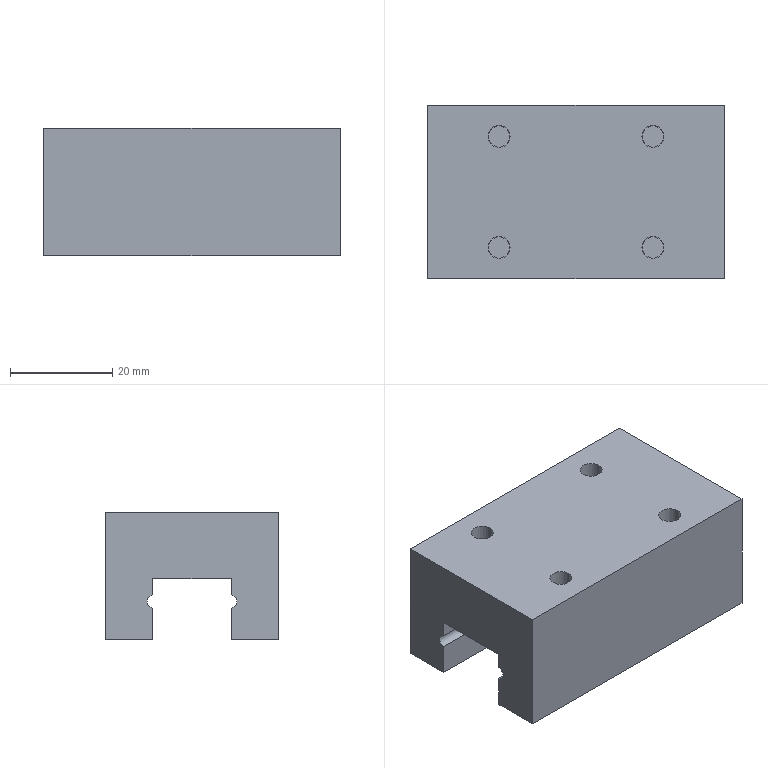Part | SolidWorks | features BaseBody 1 | 1 solid | 38 faces | box 58 x 34 x 25 mm | volume 37485 mm3 | plane 20 | cylinder 18 | commonest cylinder face diameters 4.2 x8 4.3 x8 2.6 x2
STEP:
#1=CARTESIAN_POINT('',(12.93,10.88,21.8));
#2=VERTEX_POINT('',#1);
#3=CARTESIAN_POINT('',(17.23,10.88,21.8));
#4=VERTEX_POINT('',#3);
#5=CARTESIAN_POINT('',(15.08,10.88,21.8));
#6=DIRECTION('',(0.,0.,1.));
#7=DIRECTION('',(1.,0.,0.));
#8=AXIS2_PLACEMENT_3D('',#5,#6,#7);
#9=CIRCLE('',#8,2.15);
#10=EDGE_CURVE('',#2,#4,#9,.T.);
#11=ORIENTED_EDGE('',*,*,#10,.F.);
#12=CARTESIAN_POINT('',(12.93,10.88,28.));
#13=VERTEX_POINT('',#12);
#14=CARTESIAN_POINT('',(12.93,10.88,21.8));
#15=DIRECTION('',(0.,0.,1.));
#16=VECTOR('',#15,1000.);
#17=LINE('',#14,#16);
#18=EDGE_CURVE('',#2,#13,#17,.T.);
#19=ORIENTED_EDGE('',*,*,#18,.T.);
#20=CARTESIAN_POINT('',(17.23,10.88,28.));
#21=VERTEX_POINT('',#20);
#22=CARTESIAN_POINT('',(15.08,10.88,28.));
#23=DIRECTION('',(0.,0.,-1.));
#24=DIRECTION('',(1.,0.,0.));
#25=AXIS2_PLACEMENT_3D('',#22,#23,#24);
#26=CIRCLE('',#25,2.15);
#27=EDGE_CURVE('',#21,#13,#26,.T.);
#28=ORIENTED_EDGE('',*,*,#27,.F.);
#29=CARTESIAN_POINT('',(17.23,10.88,21.8));
#30=DIRECTION('',(0.,0.,1.));
#31=VECTOR('',#30,1000.);
#32=LINE('',#29,#31);
#33=EDGE_CURVE('',#4,#21,#32,.T.);
#34=ORIENTED_EDGE('',*,*,#33,.F.);
#35=EDGE_LOOP('',(#11,#19,#28,#34));
#36=FACE_OUTER_BOUND('',#35,.T.);
#37=CARTESIAN_POINT('',(15.08,10.88,21.8));
#38=DIRECTION('',(0.,0.,1.));
#39=DIRECTION('',(1.,0.,0.));
#40=AXIS2_PLACEMENT_3D('',#37,#38,#39);
#41=CYLINDRICAL_SURFACE('',#40,2.15);
#42=ADVANCED_FACE('',(#36),#41,.F.);
#43=CARTESIAN_POINT('',(-17.23,10.88,21.8));
#44=VERTEX_POINT('',#43);
#45=CARTESIAN_POINT('',(-12.93,10.88,21.8));
#46=VERTEX_POINT('',#45);
#47=CARTESIAN_POINT('',(-15.08,10.88,21.8));
#48=DIRECTION('',(0.,0.,1.));
#49=DIRECTION('',(1.,0.,0.));
#50=AXIS2_PLACEMENT_3D('',#47,#48,#49);
#51=CIRCLE('',#50,2.15);
#52=EDGE_CURVE('',#44,#46,#51,.T.);
#53=ORIENTED_EDGE('',*,*,#52,.F.);
#54=CARTESIAN_POINT('',(-17.23,10.88,28.));
#55=VERTEX_POINT('',#54);
#56=CARTESIAN_POINT('',(-17.23,10.88,21.8));
#57=DIRECTION('',(0.,0.,1.));
#58=VECTOR('',#57,1000.);
#59=LINE('',#56,#58);
#60=EDGE_CURVE('',#44,#55,#59,.T.);
#61=ORIENTED_EDGE('',*,*,#60,.T.);
#62=CARTESIAN_POINT('',(-12.93,10.88,28.));
#63=VERTEX_POINT('',#62);
#64=CARTESIAN_POINT('',(-15.08,10.88,28.));
#65=DIRECTION('',(0.,0.,-1.));
#66=DIRECTION('',(1.,0.,0.));
#67=AXIS2_PLACEMENT_3D('',#64,#65,#66);
#68=CIRCLE('',#67,2.15);
#69=EDGE_CURVE('',#63,#55,#68,.T.);
#70=ORIENTED_EDGE('',*,*,#69,.F.);
#71=CARTESIAN_POINT('',(-12.93,10.88,21.8));
#72=DIRECTION('',(0.,0.,1.));
#73=VECTOR('',#72,1000.);
#74=LINE('',#71,#73);
#75=EDGE_CURVE('',#46,#63,#74,.T.);
#76=ORIENTED_EDGE('',*,*,#75,.F.);
#77=EDGE_LOOP('',(#53,#61,#70,#76));
#78=FACE_OUTER_BOUND('',#77,.T.);
#79=CARTESIAN_POINT('',(-15.08,10.88,21.8));
#80=DIRECTION('',(0.,0.,1.));
#81=DIRECTION('',(1.,0.,0.));
#82=AXIS2_PLACEMENT_3D('',#79,#80,#81);
#83=CYLINDRICAL_SURFACE('',#82,2.15);
#84=ADVANCED_FACE('',(#78),#83,.F.);
#85=CARTESIAN_POINT('',(12.93,-10.88,21.8));
#86=VERTEX_POINT('',#85);
#87=CARTESIAN_POINT('',(17.23,-10.88,21.8));
#88=VERTEX_POINT('',#87);
#89=CARTESIAN_POINT('',(15.08,-10.88,21.8));
#90=DIRECTION('',(0.,0.,1.));
#91=DIRECTION('',(1.,0.,0.));
#92=AXIS2_PLACEMENT_3D('',#89,#90,#91);
#93=CIRCLE('',#92,2.15);
#94=EDGE_CURVE('',#86,#88,#93,.T.);
#95=ORIENTED_EDGE('',*,*,#94,.F.);
#96=CARTESIAN_POINT('',(12.93,-10.88,28.));
#97=VERTEX_POINT('',#96);
#98=CARTESIAN_POINT('',(12.93,-10.88,21.8));
#99=DIRECTION('',(0.,0.,1.));
#100=VECTOR('',#99,1000.);
#101=LINE('',#98,#100);
#102=EDGE_CURVE('',#86,#97,#101,.T.);
#103=ORIENTED_EDGE('',*,*,#102,.T.);
#104=CARTESIAN_POINT('',(17.23,-10.88,28.));
#105=VERTEX_POINT('',#104);
#106=CARTESIAN_POINT('',(15.08,-10.88,28.));
#107=DIRECTION('',(0.,0.,-1.));
#108=DIRECTION('',(1.,0.,0.));
#109=AXIS2_PLACEMENT_3D('',#106,#107,#108);
#110=CIRCLE('',#109,2.15);
#111=EDGE_CURVE('',#105,#97,#110,.T.);
#112=ORIENTED_EDGE('',*,*,#111,.F.);
#113=CARTESIAN_POINT('',(17.23,-10.88,21.8));
#114=DIRECTION('',(0.,0.,1.));
#115=VECTOR('',#114,1000.);
#116=LINE('',#113,#115);
#117=EDGE_CURVE('',#88,#105,#116,.T.);
#118=ORIENTED_EDGE('',*,*,#117,.F.);
#119=EDGE_LOOP('',(#95,#103,#112,#118));
#120=FACE_OUTER_BOUND('',#119,.T.);
#121=CARTESIAN_POINT('',(15.08,-10.88,21.8));
#122=DIRECTION('',(0.,0.,1.));
#123=DIRECTION('',(1.,0.,0.));
#124=AXIS2_PLACEMENT_3D('',#121,#122,#123);
#125=CYLINDRICAL_SURFACE('',#124,2.15);
#126=ADVANCED_FACE('',(#120),#125,.F.);
#127=CARTESIAN_POINT('',(-17.23,-10.88,21.8));
#128=VERTEX_POINT('',#127);
#129=CARTESIAN_POINT('',(-12.93,-10.88,21.8));
#130=VERTEX_POINT('',#129);
#131=CARTESIAN_POINT('',(-15.08,-10.88,21.8));
#132=DIRECTION('',(0.,0.,1.));
#133=DIRECTION('',(1.,0.,0.));
#134=AXIS2_PLACEMENT_3D('',#131,#132,#133);
#135=CIRCLE('',#134,2.15);
#136=EDGE_CURVE('',#128,#130,#135,.T.);
#137=ORIENTED_EDGE('',*,*,#136,.F.);
#138=CARTESIAN_POINT('',(-17.23,-10.88,28.));
#139=VERTEX_POINT('',#138);
#140=CARTESIAN_POINT('',(-17.23,-10.88,21.8));
#141=DIRECTION('',(0.,0.,1.));
#142=VECTOR('',#141,1000.);
#143=LINE('',#140,#142);
#144=EDGE_CURVE('',#128,#139,#143,.T.);
#145=ORIENTED_EDGE('',*,*,#144,.T.);
#146=CARTESIAN_POINT('',(-12.93,-10.88,28.));
#147=VERTEX_POINT('',#146);
#148=CARTESIAN_POINT('',(-15.08,-10.88,28.));
#149=DIRECTION('',(0.,0.,-1.));
#150=DIRECTION('',(1.,0.,0.));
#151=AXIS2_PLACEMENT_3D('',#148,#149,#150);
#152=CIRCLE('',#151,2.15);
#153=EDGE_CURVE('',#147,#139,#152,.T.);
#154=ORIENTED_EDGE('',*,*,#153,.F.);
#155=CARTESIAN_POINT('',(-12.93,-10.88,21.8));
#156=DIRECTION('',(0.,0.,1.));
#157=VECTOR('',#156,1000.);
#158=LINE('',#155,#157);
#159=EDGE_CURVE('',#130,#147,#158,.T.);
#160=ORIENTED_EDGE('',*,*,#159,.F.);
#161=EDGE_LOOP('',(#137,#145,#154,#160));
#162=FACE_OUTER_BOUND('',#161,.T.);
#163=CARTESIAN_POINT('',(-15.08,-10.88,21.8));
#164=DIRECTION('',(0.,0.,1.));
#165=DIRECTION('',(1.,0.,0.));
#166=AXIS2_PLACEMENT_3D('',#163,#164,#165);
#167=CYLINDRICAL_SURFACE('',#166,2.15);
#168=ADVANCED_FACE('',(#162),#167,.F.);
#169=CARTESIAN_POINT('',(12.98,10.88,12.));
#170=VERTEX_POINT('',#169);
#171=CARTESIAN_POINT('',(17.18,10.88,12.));
#172=VERTEX_POINT('',#171);
#173=CARTESIAN_POINT('',(15.08,10.88,12.));
#174=DIRECTION('',(0.,0.,1.));
#175=DIRECTION('',(1.,0.,0.));
#176=AXIS2_PLACEMENT_3D('',#173,#174,#175);
#177=CIRCLE('',#176,2.1);
#178=EDGE_CURVE('',#170,#172,#177,.T.);
#179=ORIENTED_EDGE('',*,*,#178,.F.);
#180=CARTESIAN_POINT('',(12.98,10.88,21.8));
#181=VERTEX_POINT('',#180);
#182=CARTESIAN_POINT('',(12.98,10.88,12.));
#183=DIRECTION('',(0.,0.,1.));
#184=VECTOR('',#183,1000.);
#185=LINE('',#182,#184);
#186=EDGE_CURVE('',#170,#181,#185,.T.);
#187=ORIENTED_EDGE('',*,*,#186,.T.);
#188=CARTESIAN_POINT('',(17.18,10.88,21.8));
#189=VERTEX_POINT('',#188);
#190=CARTESIAN_POINT('',(15.08,10.88,21.8));
#191=DIRECTION('',(0.,0.,-1.));
#192=DIRECTION('',(1.,0.,0.));
#193=AXIS2_PLACEMENT_3D('',#190,#191,#192);
#194=CIRCLE('',#193,2.1);
#195=EDGE_CURVE('',#189,#181,#194,.T.);
#196=ORIENTED_EDGE('',*,*,#195,.F.);
#197=CARTESIAN_POINT('',(17.18,10.88,12.));
#198=DIRECTION('',(0.,0.,1.));
#199=VECTOR('',#198,1000.);
#200=LINE('',#197,#199);
#201=EDGE_CURVE('',#172,#189,#200,.T.);
#202=ORIENTED_EDGE('',*,*,#201,.F.);
#203=EDGE_LOOP('',(#179,#187,#196,#202));
#204=FACE_OUTER_BOUND('',#203,.T.);
#205=CARTESIAN_POINT('',(15.08,10.88,12.));
#206=DIRECTION('',(0.,0.,1.));
#207=DIRECTION('',(1.,0.,0.));
#208=AXIS2_PLACEMENT_3D('',#205,#206,#207);
#209=CYLINDRICAL_SURFACE('',#208,2.1);
#210=ADVANCED_FACE('',(#204),#209,.F.);
#211=CARTESIAN_POINT('',(-17.18,10.88,12.));
#212=VERTEX_POINT('',#211);
#213=CARTESIAN_POINT('',(-12.98,10.88,12.));
#214=VERTEX_POINT('',#213);
#215=CARTESIAN_POINT('',(-15.08,10.88,12.));
#216=DIRECTION('',(0.,0.,1.));
#217=DIRECTION('',(1.,0.,0.));
#218=AXIS2_PLACEMENT_3D('',#215,#216,#217);
#219=CIRCLE('',#218,2.1);
#220=EDGE_CURVE('',#212,#214,#219,.T.);
#221=ORIENTED_EDGE('',*,*,#220,.F.);
#222=CARTESIAN_POINT('',(-17.18,10.88,21.8));
#223=VERTEX_POINT('',#222);
#224=CARTESIAN_POINT('',(-17.18,10.88,12.));
#225=DIRECTION('',(0.,0.,1.));
#226=VECTOR('',#225,1000.);
#227=LINE('',#224,#226);
#228=EDGE_CURVE('',#212,#223,#227,.T.);
#229=ORIENTED_EDGE('',*,*,#228,.T.);
#230=CARTESIAN_POINT('',(-12.98,10.88,21.8));
#231=VERTEX_POINT('',#230);
#232=CARTESIAN_POINT('',(-15.08,10.88,21.8));
#233=DIRECTION('',(0.,0.,-1.));
#234=DIRECTION('',(1.,0.,0.));
#235=AXIS2_PLACEMENT_3D('',#232,#233,#234);
#236=CIRCLE('',#235,2.1);
#237=EDGE_CURVE('',#231,#223,#236,.T.);
#238=ORIENTED_EDGE('',*,*,#237,.F.);
#239=CARTESIAN_POINT('',(-12.98,10.88,12.));
#240=DIRECTION('',(0.,0.,1.));
#241=VECTOR('',#240,1000.);
#242=LINE('',#239,#241);
#243=EDGE_CURVE('',#214,#231,#242,.T.);
#244=ORIENTED_EDGE('',*,*,#243,.F.);
#245=EDGE_LOOP('',(#221,#229,#238,#244));
#246=FACE_OUTER_BOUND('',#245,.T.);
#247=CARTESIAN_POINT('',(-15.08,10.88,12.));
#248=DIRECTION('',(0.,0.,1.));
#249=DIRECTION('',(1.,0.,0.));
#250=AXIS2_PLACEMENT_3D('',#247,#248,#249);
#251=CYLINDRICAL_SURFACE('',#250,2.1);
#252=ADVANCED_FACE('',(#246),#251,.F.);
#253=CARTESIAN_POINT('',(12.98,-10.88,12.));
#254=VERTEX_POINT('',#253);
#255=CARTESIAN_POINT('',(17.18,-10.88,12.));
#256=VERTEX_POINT('',#255);
#257=CARTESIAN_POINT('',(15.08,-10.88,12.));
#258=DIRECTION('',(0.,0.,1.));
#259=DIRECTION('',(1.,0.,0.));
#260=AXIS2_PLACEMENT_3D('',#257,#258,#259);
#261=CIRCLE('',#260,2.1);
#262=EDGE_CURVE('',#254,#256,#261,.T.);
#263=ORIENTED_EDGE('',*,*,#262,.F.);
#264=CARTESIAN_POINT('',(12.98,-10.88,21.8));
#265=VERTEX_POINT('',#264);
#266=CARTESIAN_POINT('',(12.98,-10.88,12.));
#267=DIRECTION('',(0.,0.,1.));
#268=VECTOR('',#267,1000.);
#269=LINE('',#266,#268);
#270=EDGE_CURVE('',#254,#265,#269,.T.);
#271=ORIENTED_EDGE('',*,*,#270,.T.);
#272=CARTESIAN_POINT('',(17.18,-10.88,21.8));
#273=VERTEX_POINT('',#272);
#274=CARTESIAN_POINT('',(15.08,-10.88,21.8));
#275=DIRECTION('',(0.,0.,-1.));
#276=DIRECTION('',(1.,0.,0.));
#277=AXIS2_PLACEMENT_3D('',#274,#275,#276);
#278=CIRCLE('',#277,2.1);
#279=EDGE_CURVE('',#273,#265,#278,.T.);
#280=ORIENTED_EDGE('',*,*,#279,.F.);
#281=CARTESIAN_POINT('',(17.18,-10.88,12.));
#282=DIRECTION('',(0.,0.,1.));
#283=VECTOR('',#282,1000.);
#284=LINE('',#281,#283);
#285=EDGE_CURVE('',#256,#273,#284,.T.);
#286=ORIENTED_EDGE('',*,*,#285,.F.);
#287=EDGE_LOOP('',(#263,#271,#280,#286));
#288=FACE_OUTER_BOUND('',#287,.T.);
#289=CARTESIAN_POINT('',(15.08,-10.88,12.));
#290=DIRECTION('',(0.,0.,1.));
#291=DIRECTION('',(1.,0.,0.));
#292=AXIS2_PLACEMENT_3D('',#289,#290,#291);
#293=CYLINDRICAL_SURFACE('',#292,2.1);
#294=ADVANCED_FACE('',(#288),#293,.F.);
#295=CARTESIAN_POINT('',(-17.18,-10.88,12.));
#296=VERTEX_POINT('',#295);
#297=CARTESIAN_POINT('',(-12.98,-10.88,12.));
#298=VERTEX_POINT('',#297);
#299=CARTESIAN_POINT('',(-15.08,-10.88,12.));
#300=DIRECTION('',(0.,0.,1.));
#301=DIRECTION('',(1.,0.,0.));
#302=AXIS2_PLACEMENT_3D('',#299,#300,#301);
#303=CIRCLE('',#302,2.1);
#304=EDGE_CURVE('',#296,#298,#303,.T.);
#305=ORIENTED_EDGE('',*,*,#304,.F.);
#306=CARTESIAN_POINT('',(-17.18,-10.88,21.8));
#307=VERTEX_POINT('',#306);
#308=CARTESIAN_POINT('',(-17.18,-10.88,12.));
#309=DIRECTION('',(0.,0.,1.));
#310=VECTOR('',#309,1000.);
#311=LINE('',#308,#310);
#312=EDGE_CURVE('',#296,#307,#311,.T.);
#313=ORIENTED_EDGE('',*,*,#312,.T.);
#314=CARTESIAN_POINT('',(-12.98,-10.88,21.8));
#315=VERTEX_POINT('',#314);
#316=CARTESIAN_POINT('',(-15.08,-10.88,21.8));
#317=DIRECTION('',(0.,0.,-1.));
#318=DIRECTION('',(1.,0.,0.));
#319=AXIS2_PLACEMENT_3D('',#316,#317,#318);
#320=CIRCLE('',#319,2.1);
#321=EDGE_CURVE('',#315,#307,#320,.T.);
#322=ORIENTED_EDGE('',*,*,#321,.F.);
#323=CARTESIAN_POINT('',(-12.98,-10.88,12.));
#324=DIRECTION('',(0.,0.,1.));
#325=VECTOR('',#324,1000.);
#326=LINE('',#323,#325);
#327=EDGE_CURVE('',#298,#315,#326,.T.);
#328=ORIENTED_EDGE('',*,*,#327,.F.);
#329=EDGE_LOOP('',(#305,#313,#322,#328));
#330=FACE_OUTER_BOUND('',#329,.T.);
#331=CARTESIAN_POINT('',(-15.08,-10.88,12.));
#332=DIRECTION('',(0.,0.,1.));
#333=DIRECTION('',(1.,0.,0.));
#334=AXIS2_PLACEMENT_3D('',#331,#332,#333);
#335=CYLINDRICAL_SURFACE('',#334,2.1);
#336=ADVANCED_FACE('',(#330),#335,.F.);
#337=ORIENTED_EDGE('',*,*,#27,.T.);
#338=CARTESIAN_POINT('',(15.08,10.88,28.));
#339=DIRECTION('',(0.,0.,-1.));
#340=DIRECTION('',(1.,0.,0.));
#341=AXIS2_PLACEMENT_3D('',#338,#339,#340);
#342=CIRCLE('',#341,2.15);
#343=EDGE_CURVE('',#13,#21,#342,.T.);
#344=ORIENTED_EDGE('',*,*,#343,.T.);
#345=EDGE_LOOP('',(#337,#344));
#346=FACE_BOUND('',#345,.T.);
#347=ORIENTED_EDGE('',*,*,#69,.T.);
#348=CARTESIAN_POINT('',(-15.08,10.88,28.));
#349=DIRECTION('',(0.,0.,-1.));
#350=DIRECTION('',(1.,0.,0.));
#351=AXIS2_PLACEMENT_3D('',#348,#349,#350);
#352=CIRCLE('',#351,2.15);
#353=EDGE_CURVE('',#55,#63,#352,.T.);
#354=ORIENTED_EDGE('',*,*,#353,.T.);
#355=EDGE_LOOP('',(#347,#354));
#356=FACE_BOUND('',#355,.T.);
#357=ORIENTED_EDGE('',*,*,#111,.T.);
#358=CARTESIAN_POINT('',(15.08,-10.88,28.));
#359=DIRECTION('',(0.,0.,-1.));
#360=DIRECTION('',(1.,0.,0.));
#361=AXIS2_PLACEMENT_3D('',#358,#359,#360);
#362=CIRCLE('',#361,2.15);
#363=EDGE_CURVE('',#97,#105,#362,.T.);
#364=ORIENTED_EDGE('',*,*,#363,.T.);
#365=EDGE_LOOP('',(#357,#364));
#366=FACE_BOUND('',#365,.T.);
#367=ORIENTED_EDGE('',*,*,#153,.T.);
#368=CARTESIAN_POINT('',(-15.08,-10.88,28.));
#369=DIRECTION('',(0.,0.,-1.));
#370=DIRECTION('',(1.,0.,0.));
#371=AXIS2_PLACEMENT_3D('',#368,#369,#370);
#372=CIRCLE('',#371,2.15);
#373=EDGE_CURVE('',#139,#147,#372,.T.);
#374=ORIENTED_EDGE('',*,*,#373,.T.);
#375=EDGE_LOOP('',(#367,#374));
#376=FACE_BOUND('',#375,.T.);
#377=CARTESIAN_POINT('',(29.,-17.,28.));
#378=VERTEX_POINT('',#377);
#379=CARTESIAN_POINT('',(29.,17.,28.));
#380=VERTEX_POINT('',#379);
#381=CARTESIAN_POINT('',(29.,-17.,28.));
#382=DIRECTION('',(0.,1.,0.));
#383=VECTOR('',#382,1000.);
#384=LINE('',#381,#383);
#385=EDGE_CURVE('',#378,#380,#384,.T.);
#386=ORIENTED_EDGE('',*,*,#385,.T.);
#387=CARTESIAN_POINT('',(-29.,17.,28.));
#388=VERTEX_POINT('',#387);
#389=CARTESIAN_POINT('',(-29.,17.,28.));
#390=DIRECTION('',(-1.,0.,0.));
#391=VECTOR('',#390,1000.);
#392=LINE('',#389,#391);
#393=EDGE_CURVE('',#380,#388,#392,.T.);
#394=ORIENTED_EDGE('',*,*,#393,.T.);
#395=CARTESIAN_POINT('',(-29.,-17.,28.));
#396=VERTEX_POINT('',#395);
#397=CARTESIAN_POINT('',(-29.,-17.,28.));
#398=DIRECTION('',(0.,-1.,0.));
#399=VECTOR('',#398,1000.);
#400=LINE('',#397,#399);
#401=EDGE_CURVE('',#388,#396,#400,.T.);
#402=ORIENTED_EDGE('',*,*,#401,.T.);
#403=CARTESIAN_POINT('',(-29.,-17.,28.));
#404=DIRECTION('',(1.,0.,0.));
#405=VECTOR('',#404,1000.);
#406=LINE('',#403,#405);
#407=EDGE_CURVE('',#396,#378,#406,.T.);
#408=ORIENTED_EDGE('',*,*,#407,.T.);
#409=EDGE_LOOP('',(#386,#394,#402,#408));
#410=FACE_OUTER_BOUND('',#409,.T.);
#411=CARTESIAN_POINT('',(-29.,-17.,28.));
#412=DIRECTION('',(0.,0.,1.));
#413=DIRECTION('',(1.,0.,0.));
#414=AXIS2_PLACEMENT_3D('',#411,#412,#413);
#415=PLANE('',#414);
#416=ADVANCED_FACE('',(#346,#356,#366,#376,#410),#415,.T.);
#417=ORIENTED_EDGE('',*,*,#18,.F.);
#418=CARTESIAN_POINT('',(15.08,10.88,21.8));
#419=DIRECTION('',(0.,0.,1.));
#420=DIRECTION('',(1.,0.,0.));
#421=AXIS2_PLACEMENT_3D('',#418,#419,#420);
#422=CIRCLE('',#421,2.15);
#423=EDGE_CURVE('',#4,#2,#422,.T.);
#424=ORIENTED_EDGE('',*,*,#423,.F.);
#425=ORIENTED_EDGE('',*,*,#33,.T.);
#426=ORIENTED_EDGE('',*,*,#343,.F.);
#427=EDGE_LOOP('',(#417,#424,#425,#426));
#428=FACE_OUTER_BOUND('',#427,.T.);
#429=CARTESIAN_POINT('',(15.08,10.88,21.8));
#430=DIRECTION('',(0.,0.,1.));
#431=DIRECTION('',(1.,0.,0.));
#432=AXIS2_PLACEMENT_3D('',#429,#430,#431);
#433=CYLINDRICAL_SURFACE('',#432,2.15);
#434=ADVANCED_FACE('',(#428),#433,.F.);
#435=ORIENTED_EDGE('',*,*,#60,.F.);
#436=CARTESIAN_POINT('',(-15.08,10.88,21.8));
#437=DIRECTION('',(0.,0.,1.));
#438=DIRECTION('',(1.,0.,0.));
#439=AXIS2_PLACEMENT_3D('',#436,#437,#438);
#440=CIRCLE('',#439,2.15);
#441=EDGE_CURVE('',#46,#44,#440,.T.);
#442=ORIENTED_EDGE('',*,*,#441,.F.);
#443=ORIENTED_EDGE('',*,*,#75,.T.);
#444=ORIENTED_EDGE('',*,*,#353,.F.);
#445=EDGE_LOOP('',(#435,#442,#443,#444));
#446=FACE_OUTER_BOUND('',#445,.T.);
#447=CARTESIAN_POINT('',(-15.08,10.88,21.8));
#448=DIRECTION('',(0.,0.,1.));
#449=DIRECTION('',(1.,0.,0.));
#450=AXIS2_PLACEMENT_3D('',#447,#448,#449);
#451=CYLINDRICAL_SURFACE('',#450,2.15);
#452=ADVANCED_FACE('',(#446),#451,.F.);
#453=ORIENTED_EDGE('',*,*,#102,.F.);
#454=CARTESIAN_POINT('',(15.08,-10.88,21.8));
#455=DIRECTION('',(0.,0.,1.));
#456=DIRECTION('',(1.,0.,0.));
#457=AXIS2_PLACEMENT_3D('',#454,#455,#456);
#458=CIRCLE('',#457,2.15);
#459=EDGE_CURVE('',#88,#86,#458,.T.);
#460=ORIENTED_EDGE('',*,*,#459,.F.);
#461=ORIENTED_EDGE('',*,*,#117,.T.);
#462=ORIENTED_EDGE('',*,*,#363,.F.);
#463=EDGE_LOOP('',(#453,#460,#461,#462));
#464=FACE_OUTER_BOUND('',#463,.T.);
#465=CARTESIAN_POINT('',(15.08,-10.88,21.8));
#466=DIRECTION('',(0.,0.,1.));
#467=DIRECTION('',(1.,0.,0.));
#468=AXIS2_PLACEMENT_3D('',#465,#466,#467);
#469=CYLINDRICAL_SURFACE('',#468,2.15);
#470=ADVANCED_FACE('',(#464),#469,.F.);
#471=ORIENTED_EDGE('',*,*,#144,.F.);
#472=CARTESIAN_POINT('',(-15.08,-10.88,21.8));
#473=DIRECTION('',(0.,0.,1.));
#474=DIRECTION('',(1.,0.,0.));
#475=AXIS2_PLACEMENT_3D('',#472,#473,#474);
#476=CIRCLE('',#475,2.15);
#477=EDGE_CURVE('',#130,#128,#476,.T.);
#478=ORIENTED_EDGE('',*,*,#477,.F.);
#479=ORIENTED_EDGE('',*,*,#159,.T.);
#480=ORIENTED_EDGE('',*,*,#373,.F.);
#481=EDGE_LOOP('',(#471,#478,#479,#480));
#482=FACE_OUTER_BOUND('',#481,.T.);
#483=CARTESIAN_POINT('',(-15.08,-10.88,21.8));
#484=DIRECTION('',(0.,0.,1.));
#485=DIRECTION('',(1.,0.,0.));
#486=AXIS2_PLACEMENT_3D('',#483,#484,#485);
#487=CYLINDRICAL_SURFACE('',#486,2.15);
#488=ADVANCED_FACE('',(#482),#487,.F.);
#489=ORIENTED_EDGE('',*,*,#393,.F.);
#490=CARTESIAN_POINT('',(29.,17.,3.));
#491=VERTEX_POINT('',#490);
#492=CARTESIAN_POINT('',(29.,17.,3.));
#493=DIRECTION('',(0.,0.,-1.));
#494=VECTOR('',#493,1000.);
#495=LINE('',#492,#494);
#496=EDGE_CURVE('',#380,#491,#495,.T.);
#497=ORIENTED_EDGE('',*,*,#496,.T.);
#498=CARTESIAN_POINT('',(-29.,17.,3.));
#499=VERTEX_POINT('',#498);
#500=CARTESIAN_POINT('',(-29.,17.,3.));
#501=DIRECTION('',(-1.,0.,0.));
#502=VECTOR('',#501,1000.);
#503=LINE('',#500,#502);
#504=EDGE_CURVE('',#491,#499,#503,.T.);
#505=ORIENTED_EDGE('',*,*,#504,.T.);
#506=CARTESIAN_POINT('',(-29.,17.,3.));
#507=DIRECTION('',(0.,0.,1.));
#508=VECTOR('',#507,1000.);
#509=LINE('',#506,#508);
#510=EDGE_CURVE('',#499,#388,#509,.T.);
#511=ORIENTED_EDGE('',*,*,#510,.T.);
#512=EDGE_LOOP('',(#489,#497,#505,#511));
#513=FACE_OUTER_BOUND('',#512,.T.);
#514=CARTESIAN_POINT('',(-29.,17.,3.));
#515=DIRECTION('',(0.,1.,0.));
#516=DIRECTION('',(0.,0.,1.));
#517=AXIS2_PLACEMENT_3D('',#514,#515,#516);
#518=PLANE('',#517);
#519=ADVANCED_FACE('',(#513),#518,.T.);
#520=CARTESIAN_POINT('',(29.,7.65,9.209));
#521=VERTEX_POINT('',#520);
#522=CARTESIAN_POINT('',(29.,7.65,3.));
#523=VERTEX_POINT('',#522);
#524=CARTESIAN_POINT('',(29.,7.65,3.));
#525=DIRECTION('',(0.,0.,-1.));
#526=VECTOR('',#525,1000.);
#527=LINE('',#524,#526);
#528=EDGE_CURVE('',#521,#523,#527,.T.);
#529=ORIENTED_EDGE('',*,*,#528,.T.);
#530=CARTESIAN_POINT('',(29.,-17.,3.));
#531=DIRECTION('',(0.,1.,0.));
#532=VECTOR('',#531,1000.);
#533=LINE('',#530,#532);
#534=EDGE_CURVE('',#523,#491,#533,.T.);
#535=ORIENTED_EDGE('',*,*,#534,.T.);
#536=ORIENTED_EDGE('',*,*,#496,.F.);
#537=ORIENTED_EDGE('',*,*,#385,.F.);
#538=CARTESIAN_POINT('',(29.,-17.,3.));
#539=VERTEX_POINT('',#538);
#540=CARTESIAN_POINT('',(29.,-17.,3.));
#541=DIRECTION('',(0.,0.,-1.));
#542=VECTOR('',#541,1000.);
#543=LINE('',#540,#542);
#544=EDGE_CURVE('',#378,#539,#543,.T.);
#545=ORIENTED_EDGE('',*,*,#544,.T.);
#546=CARTESIAN_POINT('',(29.,-7.65,3.));
#547=VERTEX_POINT('',#546);
#548=CARTESIAN_POINT('',(29.,-17.,3.));
#549=DIRECTION('',(0.,1.,0.));
#550=VECTOR('',#549,1000.);
#551=LINE('',#548,#550);
#552=EDGE_CURVE('',#539,#547,#551,.T.);
#553=ORIENTED_EDGE('',*,*,#552,.T.);
#554=CARTESIAN_POINT('',(29.,-7.65,9.209));
#555=VERTEX_POINT('',#554);
#556=CARTESIAN_POINT('',(29.,-7.65,3.));
#557=DIRECTION('',(0.,0.,1.));
#558=VECTOR('',#557,1000.);
#559=LINE('',#556,#558);
#560=EDGE_CURVE('',#547,#555,#559,.T.);
#561=ORIENTED_EDGE('',*,*,#560,.T.);
#562=CARTESIAN_POINT('',(29.,-7.65,11.791));
#563=VERTEX_POINT('',#562);
#564=CARTESIAN_POINT('',(29.,-7.5,10.5));
#565=DIRECTION('',(-1.,0.,0.));
#566=DIRECTION('',(0.,0.,-1.));
#567=AXIS2_PLACEMENT_3D('',#564,#565,#566);
#568=CIRCLE('',#567,1.3);
#569=EDGE_CURVE('',#555,#563,#568,.T.);
#570=ORIENTED_EDGE('',*,*,#569,.T.);
#571=CARTESIAN_POINT('',(29.,-7.65,15.));
#572=VERTEX_POINT('',#571);
#573=CARTESIAN_POINT('',(29.,-7.65,3.));
#574=DIRECTION('',(0.,0.,1.));
#575=VECTOR('',#574,1000.);
#576=LINE('',#573,#575);
#577=EDGE_CURVE('',#563,#572,#576,.T.);
#578=ORIENTED_EDGE('',*,*,#577,.T.);
#579=CARTESIAN_POINT('',(29.,7.65,15.));
#580=VERTEX_POINT('',#579);
#581=CARTESIAN_POINT('',(29.,-17.,15.));
#582=DIRECTION('',(0.,1.,0.));
#583=VECTOR('',#582,1000.);
#584=LINE('',#581,#583);
#585=EDGE_CURVE('',#572,#580,#584,.T.);
#586=ORIENTED_EDGE('',*,*,#585,.T.);
#587=CARTESIAN_POINT('',(29.,7.65,11.791));
#588=VERTEX_POINT('',#587);
#589=CARTESIAN_POINT('',(29.,7.65,3.));
#590=DIRECTION('',(0.,0.,-1.));
#591=VECTOR('',#590,1000.);
#592=LINE('',#589,#591);
#593=EDGE_CURVE('',#580,#588,#592,.T.);
#594=ORIENTED_EDGE('',*,*,#593,.T.);
#595=CARTESIAN_POINT('',(29.,7.5,10.5));
#596=DIRECTION('',(-1.,0.,0.));
#597=DIRECTION('',(0.,0.,-1.));
#598=AXIS2_PLACEMENT_3D('',#595,#596,#597);
#599=CIRCLE('',#598,1.3);
#600=EDGE_CURVE('',#588,#521,#599,.T.);
#601=ORIENTED_EDGE('',*,*,#600,.T.);
#602=EDGE_LOOP('',(#529,#535,#536,#537,#545,#553,#561,#570,#578,#586,#594,#601));
#603=FACE_OUTER_BOUND('',#602,.T.);
#604=CARTESIAN_POINT('',(29.,-17.,3.));
#605=DIRECTION('',(1.,0.,0.));
#606=DIRECTION('',(0.,0.,-1.));
#607=AXIS2_PLACEMENT_3D('',#604,#605,#606);
#608=PLANE('',#607);
#609=ADVANCED_FACE('',(#603),#608,.T.);
#610=ORIENTED_EDGE('',*,*,#407,.F.);
#611=CARTESIAN_POINT('',(-29.,-17.,3.));
#612=VERTEX_POINT('',#611);
#613=CARTESIAN_POINT('',(-29.,-17.,3.));
#614=DIRECTION('',(0.,0.,1.));
#615=VECTOR('',#614,1000.);
#616=LINE('',#613,#615);
#617=EDGE_CURVE('',#612,#396,#616,.T.);
#618=ORIENTED_EDGE('',*,*,#617,.F.);
#619=CARTESIAN_POINT('',(-29.,-17.,3.));
#620=DIRECTION('',(-1.,0.,0.));
#621=VECTOR('',#620,1000.);
#622=LINE('',#619,#621);
#623=EDGE_CURVE('',#539,#612,#622,.T.);
#624=ORIENTED_EDGE('',*,*,#623,.F.);
#625=ORIENTED_EDGE('',*,*,#544,.F.);
#626=EDGE_LOOP('',(#610,#618,#624,#625));
#627=FACE_OUTER_BOUND('',#626,.T.);
#628=CARTESIAN_POINT('',(-29.,-17.,3.));
#629=DIRECTION('',(0.,1.,0.));
#630=DIRECTION('',(0.,0.,1.));
#631=AXIS2_PLACEMENT_3D('',#628,#629,#630);
#632=PLANE('',#631);
#633=ADVANCED_FACE('',(#627),#632,.F.);
#634=CARTESIAN_POINT('',(-29.,7.65,9.209));
#635=VERTEX_POINT('',#634);
#636=CARTESIAN_POINT('',(-29.,7.65,3.));
#637=VERTEX_POINT('',#636);
#638=CARTESIAN_POINT('',(-29.,7.65,3.));
#639=DIRECTION('',(0.,0.,-1.));
#640=VECTOR('',#639,1000.);
#641=LINE('',#638,#640);
#642=EDGE_CURVE('',#635,#637,#641,.T.);
#643=ORIENTED_EDGE('',*,*,#642,.F.);
#644=CARTESIAN_POINT('',(-29.,7.65,11.791));
#645=VERTEX_POINT('',#644);
#646=CARTESIAN_POINT('',(-29.,7.5,10.5));
#647=DIRECTION('',(-1.,0.,0.));
#648=DIRECTION('',(0.,0.,-1.));
#649=AXIS2_PLACEMENT_3D('',#646,#647,#648);
#650=CIRCLE('',#649,1.3);
#651=EDGE_CURVE('',#645,#635,#650,.T.);
#652=ORIENTED_EDGE('',*,*,#651,.F.);
#653=CARTESIAN_POINT('',(-29.,7.65,15.));
#654=VERTEX_POINT('',#653);
#655=CARTESIAN_POINT('',(-29.,7.65,3.));
#656=DIRECTION('',(0.,0.,-1.));
#657=VECTOR('',#656,1000.);
#658=LINE('',#655,#657);
#659=EDGE_CURVE('',#654,#645,#658,.T.);
#660=ORIENTED_EDGE('',*,*,#659,.F.);
#661=CARTESIAN_POINT('',(-29.,-7.65,15.));
#662=VERTEX_POINT('',#661);
#663=CARTESIAN_POINT('',(-29.,-17.,15.));
#664=DIRECTION('',(0.,1.,0.));
#665=VECTOR('',#664,1000.);
#666=LINE('',#663,#665);
#667=EDGE_CURVE('',#662,#654,#666,.T.);
#668=ORIENTED_EDGE('',*,*,#667,.F.);
#669=CARTESIAN_POINT('',(-29.,-7.65,11.791));
#670=VERTEX_POINT('',#669);
#671=CARTESIAN_POINT('',(-29.,-7.65,3.));
#672=DIRECTION('',(0.,0.,1.));
#673=VECTOR('',#672,1000.);
#674=LINE('',#671,#673);
#675=EDGE_CURVE('',#670,#662,#674,.T.);
#676=ORIENTED_EDGE('',*,*,#675,.F.);
#677=CARTESIAN_POINT('',(-29.,-7.65,9.209));
#678=VERTEX_POINT('',#677);
#679=CARTESIAN_POINT('',(-29.,-7.5,10.5));
#680=DIRECTION('',(-1.,0.,0.));
#681=DIRECTION('',(0.,0.,-1.));
#682=AXIS2_PLACEMENT_3D('',#679,#680,#681);
#683=CIRCLE('',#682,1.3);
#684=EDGE_CURVE('',#678,#670,#683,.T.);
#685=ORIENTED_EDGE('',*,*,#684,.F.);
#686=CARTESIAN_POINT('',(-29.,-7.65,3.));
#687=VERTEX_POINT('',#686);
#688=CARTESIAN_POINT('',(-29.,-7.65,3.));
#689=DIRECTION('',(0.,0.,1.));
#690=VECTOR('',#689,1000.);
#691=LINE('',#688,#690);
#692=EDGE_CURVE('',#687,#678,#691,.T.);
#693=ORIENTED_EDGE('',*,*,#692,.F.);
#694=CARTESIAN_POINT('',(-29.,-17.,3.));
#695=DIRECTION('',(0.,1.,0.));
#696=VECTOR('',#695,1000.);
#697=LINE('',#694,#696);
#698=EDGE_CURVE('',#612,#687,#697,.T.);
#699=ORIENTED_EDGE('',*,*,#698,.F.);
#700=ORIENTED_EDGE('',*,*,#617,.T.);
#701=ORIENTED_EDGE('',*,*,#401,.F.);
#702=ORIENTED_EDGE('',*,*,#510,.F.);
#703=CARTESIAN_POINT('',(-29.,-17.,3.));
#704=DIRECTION('',(0.,1.,0.));
#705=VECTOR('',#704,1000.);
#706=LINE('',#703,#705);
#707=EDGE_CURVE('',#637,#499,#706,.T.);
#708=ORIENTED_EDGE('',*,*,#707,.F.);
#709=EDGE_LOOP('',(#643,#652,#660,#668,#676,#685,#693,#699,#700,#701,#702,#708));
#710=FACE_OUTER_BOUND('',#709,.T.);
#711=CARTESIAN_POINT('',(-29.,-17.,3.));
#712=DIRECTION('',(1.,0.,0.));
#713=DIRECTION('',(0.,0.,-1.));
#714=AXIS2_PLACEMENT_3D('',#711,#712,#713);
#715=PLANE('',#714);
#716=ADVANCED_FACE('',(#710),#715,.F.);
#717=ORIENTED_EDGE('',*,*,#195,.T.);
#718=CARTESIAN_POINT('',(15.08,10.88,21.8));
#719=DIRECTION('',(0.,0.,-1.));
#720=DIRECTION('',(1.,0.,0.));
#721=AXIS2_PLACEMENT_3D('',#718,#719,#720);
#722=CIRCLE('',#721,2.1);
#723=EDGE_CURVE('',#181,#189,#722,.T.);
#724=ORIENTED_EDGE('',*,*,#723,.T.);
#725=EDGE_LOOP('',(#717,#724));
#726=FACE_BOUND('',#725,.T.);
#727=ORIENTED_EDGE('',*,*,#423,.T.);
#728=ORIENTED_EDGE('',*,*,#10,.T.);
#729=EDGE_LOOP('',(#727,#728));
#730=FACE_OUTER_BOUND('',#729,.T.);
#731=CARTESIAN_POINT('',(15.08,10.88,21.8));
#732=DIRECTION('',(0.,0.,1.));
#733=DIRECTION('',(1.,0.,0.));
#734=AXIS2_PLACEMENT_3D('',#731,#732,#733);
#735=PLANE('',#734);
#736=ADVANCED_FACE('',(#726,#730),#735,.T.);
#737=ORIENTED_EDGE('',*,*,#237,.T.);
#738=CARTESIAN_POINT('',(-15.08,10.88,21.8));
#739=DIRECTION('',(0.,0.,-1.));
#740=DIRECTION('',(1.,0.,0.));
#741=AXIS2_PLACEMENT_3D('',#738,#739,#740);
#742=CIRCLE('',#741,2.1);
#743=EDGE_CURVE('',#223,#231,#742,.T.);
#744=ORIENTED_EDGE('',*,*,#743,.T.);
#745=EDGE_LOOP('',(#737,#744));
#746=FACE_BOUND('',#745,.T.);
#747=ORIENTED_EDGE('',*,*,#441,.T.);
#748=ORIENTED_EDGE('',*,*,#52,.T.);
#749=EDGE_LOOP('',(#747,#748));
#750=FACE_OUTER_BOUND('',#749,.T.);
#751=CARTESIAN_POINT('',(-15.08,10.88,21.8));
#752=DIRECTION('',(0.,0.,1.));
#753=DIRECTION('',(1.,0.,0.));
#754=AXIS2_PLACEMENT_3D('',#751,#752,#753);
#755=PLANE('',#754);
#756=ADVANCED_FACE('',(#746,#750),#755,.T.);
#757=ORIENTED_EDGE('',*,*,#279,.T.);
#758=CARTESIAN_POINT('',(15.08,-10.88,21.8));
#759=DIRECTION('',(0.,0.,-1.));
#760=DIRECTION('',(1.,0.,0.));
#761=AXIS2_PLACEMENT_3D('',#758,#759,#760);
#762=CIRCLE('',#761,2.1);
#763=EDGE_CURVE('',#265,#273,#762,.T.);
#764=ORIENTED_EDGE('',*,*,#763,.T.);
#765=EDGE_LOOP('',(#757,#764));
#766=FACE_BOUND('',#765,.T.);
#767=ORIENTED_EDGE('',*,*,#459,.T.);
#768=ORIENTED_EDGE('',*,*,#94,.T.);
#769=EDGE_LOOP('',(#767,#768));
#770=FACE_OUTER_BOUND('',#769,.T.);
#771=CARTESIAN_POINT('',(15.08,-10.88,21.8));
#772=DIRECTION('',(0.,0.,1.));
#773=DIRECTION('',(1.,0.,0.));
#774=AXIS2_PLACEMENT_3D('',#771,#772,#773);
#775=PLANE('',#774);
#776=ADVANCED_FACE('',(#766,#770),#775,.T.);
#777=ORIENTED_EDGE('',*,*,#321,.T.);
#778=CARTESIAN_POINT('',(-15.08,-10.88,21.8));
#779=DIRECTION('',(0.,0.,-1.));
#780=DIRECTION('',(1.,0.,0.));
#781=AXIS2_PLACEMENT_3D('',#778,#779,#780);
#782=CIRCLE('',#781,2.1);
#783=EDGE_CURVE('',#307,#315,#782,.T.);
#784=ORIENTED_EDGE('',*,*,#783,.T.);
#785=EDGE_LOOP('',(#777,#784));
#786=FACE_BOUND('',#785,.T.);
#787=ORIENTED_EDGE('',*,*,#477,.T.);
#788=ORIENTED_EDGE('',*,*,#136,.T.);
#789=EDGE_LOOP('',(#787,#788));
#790=FACE_OUTER_BOUND('',#789,.T.);
#791=CARTESIAN_POINT('',(-15.08,-10.88,21.8));
#792=DIRECTION('',(0.,0.,1.));
#793=DIRECTION('',(1.,0.,0.));
#794=AXIS2_PLACEMENT_3D('',#791,#792,#793);
#795=PLANE('',#794);
#796=ADVANCED_FACE('',(#786,#790),#795,.T.);
#797=ORIENTED_EDGE('',*,*,#534,.F.);
#798=CARTESIAN_POINT('',(-29.,7.65,3.));
#799=DIRECTION('',(1.,0.,0.));
#800=VECTOR('',#799,1000.);
#801=LINE('',#798,#800);
#802=EDGE_CURVE('',#637,#523,#801,.T.);
#803=ORIENTED_EDGE('',*,*,#802,.F.);
#804=ORIENTED_EDGE('',*,*,#707,.T.);
#805=ORIENTED_EDGE('',*,*,#504,.F.);
#806=EDGE_LOOP('',(#797,#803,#804,#805));
#807=FACE_OUTER_BOUND('',#806,.T.);
#808=CARTESIAN_POINT('',(-29.,-17.,3.));
#809=DIRECTION('',(0.,0.,1.));
#810=DIRECTION('',(1.,0.,0.));
#811=AXIS2_PLACEMENT_3D('',#808,#809,#810);
#812=PLANE('',#811);
#813=ADVANCED_FACE('',(#807),#812,.F.);
#814=ORIENTED_EDGE('',*,*,#528,.F.);
#815=CARTESIAN_POINT('',(-30.,7.65,9.209));
#816=DIRECTION('',(1.,0.,0.));
#817=VECTOR('',#816,1000.);
#818=LINE('',#815,#817);
#819=EDGE_CURVE('',#635,#521,#818,.T.);
#820=ORIENTED_EDGE('',*,*,#819,.F.);
#821=ORIENTED_EDGE('',*,*,#642,.T.);
#822=ORIENTED_EDGE('',*,*,#802,.T.);
#823=EDGE_LOOP('',(#814,#820,#821,#822));
#824=FACE_OUTER_BOUND('',#823,.T.);
#825=CARTESIAN_POINT('',(-30.,7.65,-0.3));
#826=DIRECTION('',(0.,1.,0.));
#827=DIRECTION('',(0.,0.,1.));
#828=AXIS2_PLACEMENT_3D('',#825,#826,#827);
#829=PLANE('',#828);
#830=ADVANCED_FACE('',(#824),#829,.F.);
#831=CARTESIAN_POINT('',(-30.,7.65,11.791));
#832=DIRECTION('',(1.,0.,0.));
#833=VECTOR('',#832,1000.);
#834=LINE('',#831,#833);
#835=EDGE_CURVE('',#645,#588,#834,.T.);
#836=ORIENTED_EDGE('',*,*,#835,.F.);
#837=ORIENTED_EDGE('',*,*,#651,.T.);
#838=ORIENTED_EDGE('',*,*,#819,.T.);
#839=ORIENTED_EDGE('',*,*,#600,.F.);
#840=EDGE_LOOP('',(#836,#837,#838,#839));
#841=FACE_OUTER_BOUND('',#840,.T.);
#842=CARTESIAN_POINT('',(-30.,7.5,10.5));
#843=DIRECTION('',(1.,0.,0.));
#844=DIRECTION('',(0.,0.,-1.));
#845=AXIS2_PLACEMENT_3D('',#842,#843,#844);
#846=CYLINDRICAL_SURFACE('',#845,1.3);
#847=ADVANCED_FACE('',(#841),#846,.F.);
#848=ORIENTED_EDGE('',*,*,#593,.F.);
#849=CARTESIAN_POINT('',(-30.,7.65,15.));
#850=DIRECTION('',(1.,0.,0.));
#851=VECTOR('',#850,1000.);
#852=LINE('',#849,#851);
#853=EDGE_CURVE('',#654,#580,#852,.T.);
#854=ORIENTED_EDGE('',*,*,#853,.F.);
#855=ORIENTED_EDGE('',*,*,#659,.T.);
#856=ORIENTED_EDGE('',*,*,#835,.T.);
#857=EDGE_LOOP('',(#848,#854,#855,#856));
#858=FACE_OUTER_BOUND('',#857,.T.);
#859=CARTESIAN_POINT('',(-30.,7.65,-0.3));
#860=DIRECTION('',(0.,1.,0.));
#861=DIRECTION('',(0.,0.,1.));
#862=AXIS2_PLACEMENT_3D('',#859,#860,#861);
#863=PLANE('',#862);
#864=ADVANCED_FACE('',(#858),#863,.F.);
#865=CARTESIAN_POINT('',(-30.,-7.65,15.));
#866=DIRECTION('',(1.,0.,0.));
#867=VECTOR('',#866,1000.);
#868=LINE('',#865,#867);
#869=EDGE_CURVE('',#662,#572,#868,.T.);
#870=ORIENTED_EDGE('',*,*,#869,.F.);
#871=ORIENTED_EDGE('',*,*,#667,.T.);
#872=ORIENTED_EDGE('',*,*,#853,.T.);
#873=ORIENTED_EDGE('',*,*,#585,.F.);
#874=EDGE_LOOP('',(#870,#871,#872,#873));
#875=FACE_OUTER_BOUND('',#874,.T.);
#876=CARTESIAN_POINT('',(-30.,-7.65,15.));
#877=DIRECTION('',(0.,0.,1.));
#878=DIRECTION('',(1.,0.,0.));
#879=AXIS2_PLACEMENT_3D('',#876,#877,#878);
#880=PLANE('',#879);
#881=ADVANCED_FACE('',(#875),#880,.F.);
#882=ORIENTED_EDGE('',*,*,#577,.F.);
#883=CARTESIAN_POINT('',(-30.,-7.65,11.791));
#884=DIRECTION('',(-1.,0.,0.));
#885=VECTOR('',#884,1000.);
#886=LINE('',#883,#885);
#887=EDGE_CURVE('',#563,#670,#886,.T.);
#888=ORIENTED_EDGE('',*,*,#887,.T.);
#889=ORIENTED_EDGE('',*,*,#675,.T.);
#890=ORIENTED_EDGE('',*,*,#869,.T.);
#891=EDGE_LOOP('',(#882,#888,#889,#890));
#892=FACE_OUTER_BOUND('',#891,.T.);
#893=CARTESIAN_POINT('',(-30.,-7.65,-0.3));
#894=DIRECTION('',(0.,1.,0.));
#895=DIRECTION('',(0.,0.,1.));
#896=AXIS2_PLACEMENT_3D('',#893,#894,#895);
#897=PLANE('',#896);
#898=ADVANCED_FACE('',(#892),#897,.T.);
#899=CARTESIAN_POINT('',(-30.,-7.65,9.209));
#900=DIRECTION('',(1.,0.,0.));
#901=VECTOR('',#900,1000.);
#902=LINE('',#899,#901);
#903=EDGE_CURVE('',#678,#555,#902,.T.);
#904=ORIENTED_EDGE('',*,*,#903,.F.);
#905=ORIENTED_EDGE('',*,*,#684,.T.);
#906=ORIENTED_EDGE('',*,*,#887,.F.);
#907=ORIENTED_EDGE('',*,*,#569,.F.);
#908=EDGE_LOOP('',(#904,#905,#906,#907));
#909=FACE_OUTER_BOUND('',#908,.T.);
#910=CARTESIAN_POINT('',(-30.,-7.5,10.5));
#911=DIRECTION('',(1.,0.,0.));
#912=DIRECTION('',(0.,0.,-1.));
#913=AXIS2_PLACEMENT_3D('',#910,#911,#912);
#914=CYLINDRICAL_SURFACE('',#913,1.3);
#915=ADVANCED_FACE('',(#909),#914,.F.);
#916=ORIENTED_EDGE('',*,*,#560,.F.);
#917=CARTESIAN_POINT('',(-30.,-7.65,3.));
#918=DIRECTION('',(-1.,0.,0.));
#919=VECTOR('',#918,1000.);
#920=LINE('',#917,#919);
#921=EDGE_CURVE('',#547,#687,#920,.T.);
#922=ORIENTED_EDGE('',*,*,#921,.T.);
#923=ORIENTED_EDGE('',*,*,#692,.T.);
#924=ORIENTED_EDGE('',*,*,#903,.T.);
#925=EDGE_LOOP('',(#916,#922,#923,#924));
#926=FACE_OUTER_BOUND('',#925,.T.);
#927=CARTESIAN_POINT('',(-30.,-7.65,-0.3));
#928=DIRECTION('',(0.,1.,0.));
#929=DIRECTION('',(0.,0.,1.));
#930=AXIS2_PLACEMENT_3D('',#927,#928,#929);
#931=PLANE('',#930);
#932=ADVANCED_FACE('',(#926),#931,.T.);
#933=ORIENTED_EDGE('',*,*,#552,.F.);
#934=ORIENTED_EDGE('',*,*,#623,.T.);
#935=ORIENTED_EDGE('',*,*,#698,.T.);
#936=ORIENTED_EDGE('',*,*,#921,.F.);
#937=EDGE_LOOP('',(#933,#934,#935,#936));
#938=FACE_OUTER_BOUND('',#937,.T.);
#939=CARTESIAN_POINT('',(-29.,-17.,3.));
#940=DIRECTION('',(0.,0.,1.));
#941=DIRECTION('',(1.,0.,0.));
#942=AXIS2_PLACEMENT_3D('',#939,#940,#941);
#943=PLANE('',#942);
#944=ADVANCED_FACE('',(#938),#943,.F.);
#945=ORIENTED_EDGE('',*,*,#186,.F.);
#946=CARTESIAN_POINT('',(15.08,10.88,12.));
#947=DIRECTION('',(0.,0.,1.));
#948=DIRECTION('',(1.,0.,0.));
#949=AXIS2_PLACEMENT_3D('',#946,#947,#948);
#950=CIRCLE('',#949,2.1);
#951=EDGE_CURVE('',#172,#170,#950,.T.);
#952=ORIENTED_EDGE('',*,*,#951,.F.);
#953=ORIENTED_EDGE('',*,*,#201,.T.);
#954=ORIENTED_EDGE('',*,*,#723,.F.);
#955=EDGE_LOOP('',(#945,#952,#953,#954));
#956=FACE_OUTER_BOUND('',#955,.T.);
#957=CARTESIAN_POINT('',(15.08,10.88,12.));
#958=DIRECTION('',(0.,0.,1.));
#959=DIRECTION('',(1.,0.,0.));
#960=AXIS2_PLACEMENT_3D('',#957,#958,#959);
#961=CYLINDRICAL_SURFACE('',#960,2.1);
#962=ADVANCED_FACE('',(#956),#961,.F.);
#963=ORIENTED_EDGE('',*,*,#228,.F.);
#964=CARTESIAN_POINT('',(-15.08,10.88,12.));
#965=DIRECTION('',(0.,0.,1.));
#966=DIRECTION('',(1.,0.,0.));
#967=AXIS2_PLACEMENT_3D('',#964,#965,#966);
#968=CIRCLE('',#967,2.1);
#969=EDGE_CURVE('',#214,#212,#968,.T.);
#970=ORIENTED_EDGE('',*,*,#969,.F.);
#971=ORIENTED_EDGE('',*,*,#243,.T.);
#972=ORIENTED_EDGE('',*,*,#743,.F.);
#973=EDGE_LOOP('',(#963,#970,#971,#972));
#974=FACE_OUTER_BOUND('',#973,.T.);
#975=CARTESIAN_POINT('',(-15.08,10.88,12.));
#976=DIRECTION('',(0.,0.,1.));
#977=DIRECTION('',(1.,0.,0.));
#978=AXIS2_PLACEMENT_3D('',#975,#976,#977);
#979=CYLINDRICAL_SURFACE('',#978,2.1);
#980=ADVANCED_FACE('',(#974),#979,.F.);
#981=ORIENTED_EDGE('',*,*,#270,.F.);
#982=CARTESIAN_POINT('',(15.08,-10.88,12.));
#983=DIRECTION('',(0.,0.,1.));
#984=DIRECTION('',(1.,0.,0.));
#985=AXIS2_PLACEMENT_3D('',#982,#983,#984);
#986=CIRCLE('',#985,2.1);
#987=EDGE_CURVE('',#256,#254,#986,.T.);
#988=ORIENTED_EDGE('',*,*,#987,.F.);
#989=ORIENTED_EDGE('',*,*,#285,.T.);
#990=ORIENTED_EDGE('',*,*,#763,.F.);
#991=EDGE_LOOP('',(#981,#988,#989,#990));
#992=FACE_OUTER_BOUND('',#991,.T.);
#993=CARTESIAN_POINT('',(15.08,-10.88,12.));
#994=DIRECTION('',(0.,0.,1.));
#995=DIRECTION('',(1.,0.,0.));
#996=AXIS2_PLACEMENT_3D('',#993,#994,#995);
#997=CYLINDRICAL_SURFACE('',#996,2.1);
#998=ADVANCED_FACE('',(#992),#997,.F.);
#999=ORIENTED_EDGE('',*,*,#312,.F.);
#1000=CARTESIAN_POINT('',(-15.08,-10.88,12.));
#1001=DIRECTION('',(0.,0.,1.));
#1002=DIRECTION('',(1.,0.,0.));
#1003=AXIS2_PLACEMENT_3D('',#1000,#1001,#1002);
#1004=CIRCLE('',#1003,2.1);
#1005=EDGE_CURVE('',#298,#296,#1004,.T.);
#1006=ORIENTED_EDGE('',*,*,#1005,.F.);
#1007=ORIENTED_EDGE('',*,*,#327,.T.);
#1008=ORIENTED_EDGE('',*,*,#783,.F.);
#1009=EDGE_LOOP('',(#999,#1006,#1007,#1008));
#1010=FACE_OUTER_BOUND('',#1009,.T.);
#1011=CARTESIAN_POINT('',(-15.08,-10.88,12.));
#1012=DIRECTION('',(0.,0.,1.));
#1013=DIRECTION('',(1.,0.,0.));
#1014=AXIS2_PLACEMENT_3D('',#1011,#1012,#1013);
#1015=CYLINDRICAL_SURFACE('',#1014,2.1);
#1016=ADVANCED_FACE('',(#1010),#1015,.F.);
#1017=ORIENTED_EDGE('',*,*,#951,.T.);
#1018=ORIENTED_EDGE('',*,*,#178,.T.);
#1019=EDGE_LOOP('',(#1017,#1018));
#1020=FACE_OUTER_BOUND('',#1019,.T.);
#1021=CARTESIAN_POINT('',(15.08,10.88,12.));
#1022=DIRECTION('',(0.,0.,1.));
#1023=DIRECTION('',(1.,0.,0.));
#1024=AXIS2_PLACEMENT_3D('',#1021,#1022,#1023);
#1025=PLANE('',#1024);
#1026=ADVANCED_FACE('',(#1020),#1025,.T.);
#1027=ORIENTED_EDGE('',*,*,#969,.T.);
#1028=ORIENTED_EDGE('',*,*,#220,.T.);
#1029=EDGE_LOOP('',(#1027,#1028));
#1030=FACE_OUTER_BOUND('',#1029,.T.);
#1031=CARTESIAN_POINT('',(-15.08,10.88,12.));
#1032=DIRECTION('',(0.,0.,1.));
#1033=DIRECTION('',(1.,0.,0.));
#1034=AXIS2_PLACEMENT_3D('',#1031,#1032,#1033);
#1035=PLANE('',#1034);
#1036=ADVANCED_FACE('',(#1030),#1035,.T.);
#1037=ORIENTED_EDGE('',*,*,#987,.T.);
#1038=ORIENTED_EDGE('',*,*,#262,.T.);
#1039=EDGE_LOOP('',(#1037,#1038));
#1040=FACE_OUTER_BOUND('',#1039,.T.);
#1041=CARTESIAN_POINT('',(15.08,-10.88,12.));
#1042=DIRECTION('',(0.,0.,1.));
#1043=DIRECTION('',(1.,0.,0.));
#1044=AXIS2_PLACEMENT_3D('',#1041,#1042,#1043);
#1045=PLANE('',#1044);
#1046=ADVANCED_FACE('',(#1040),#1045,.T.);
#1047=ORIENTED_EDGE('',*,*,#1005,.T.);
#1048=ORIENTED_EDGE('',*,*,#304,.T.);
#1049=EDGE_LOOP('',(#1047,#1048));
#1050=FACE_OUTER_BOUND('',#1049,.T.);
#1051=CARTESIAN_POINT('',(-15.08,-10.88,12.));
#1052=DIRECTION('',(0.,0.,1.));
#1053=DIRECTION('',(1.,0.,0.));
#1054=AXIS2_PLACEMENT_3D('',#1051,#1052,#1053);
#1055=PLANE('',#1054);
#1056=ADVANCED_FACE('',(#1050),#1055,.T.);
#1057=CLOSED_SHELL('',(#42,#84,#126,#168,#210,#252,#294,#336,#416,#434,#452,#470,#488,#519,#609,#633,#716,#736,#756,#776,#796,#813,#830,#847,#864,#881,#898,#915,#932,#944,#962,#980,#998,#1016,#1026,#1036,#1046,#1056));
#1058=MANIFOLD_SOLID_BREP('',#1057);
#1059=CARTESIAN_POINT('',(0.,0.,0.));
#1060=DIRECTION('',(0.,0.,1.));
#1061=DIRECTION('',(1.,0.,0.));
#1062=AXIS2_PLACEMENT_3D('',#1059,#1060,#1061);
#1063=(LENGTH_UNIT()NAMED_UNIT(*)SI_UNIT(.MILLI.,.METRE.));
#1064=UNCERTAINTY_MEASURE_WITH_UNIT(LENGTH_MEASURE(0.00001),#1063,'','');
#1065=(NAMED_UNIT(*)PLANE_ANGLE_UNIT()SI_UNIT($,.RADIAN.));
#1066=(NAMED_UNIT(*)SI_UNIT($,.STERADIAN.)SOLID_ANGLE_UNIT());
#1067=(GEOMETRIC_REPRESENTATION_CONTEXT(3)GLOBAL_UNCERTAINTY_ASSIGNED_CONTEXT((#1064))GLOBAL_UNIT_ASSIGNED_CONTEXT((#1063,#1065,#1066))REPRESENTATION_CONTEXT('',''));
#1068=ADVANCED_BREP_SHAPE_REPRESENTATION('',(#1058,#1062),#1067);